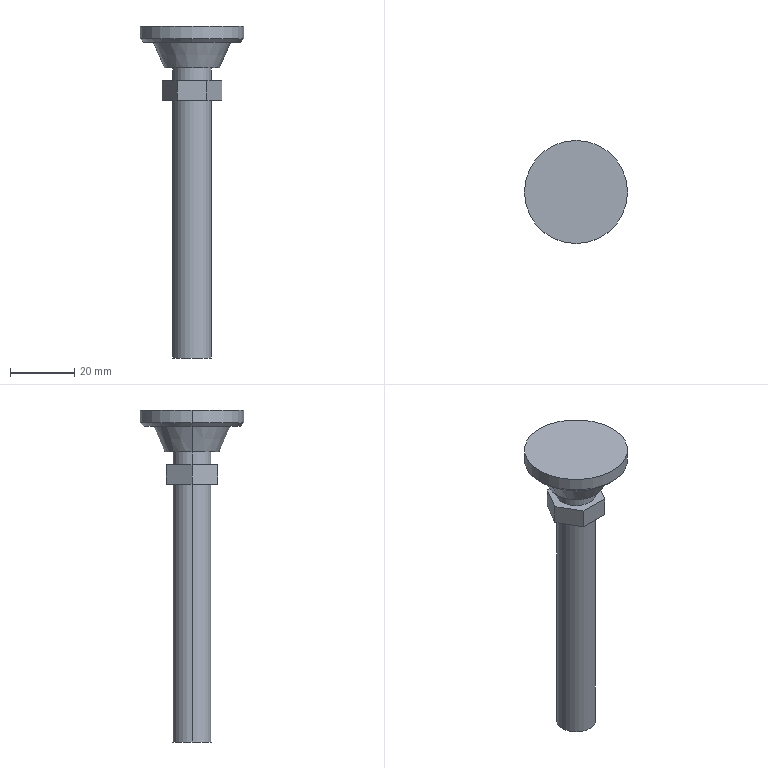Part | STEP file | 274D2D3-1.stp.STEP | 2 solids | 27 faces | box 32 x 32 x 103 mm | volume 17446 mm3 | plane 12 | cylinder 6 | cone 5 | sphere 4 | commonest cylinder face diameters 12 x4 32 x2
STEP:
#1=CARTESIAN_POINT('',(-6.1,0.,-13.));
#2=VERTEX_POINT('',#1);
#3=CARTESIAN_POINT('',(6.1,0.,-13.));
#4=VERTEX_POINT('',#3);
#5=CARTESIAN_POINT('',(0.,0.,-13.));
#6=DIRECTION('',(0.,1.,0.));
#7=DIRECTION('',(-1.,0.,0.));
#8=AXIS2_PLACEMENT_3D('',#5,#6,#7);
#9=CIRCLE('',#8,6.1);
#10=EDGE_CURVE('',#2,#4,#9,.T.);
#11=ORIENTED_EDGE('',*,*,#10,.T.);
#12=CARTESIAN_POINT('',(0.,0.,-13.));
#13=DIRECTION('',(0.,0.,-1.));
#14=DIRECTION('',(1.,0.,0.));
#15=AXIS2_PLACEMENT_3D('',#12,#13,#14);
#16=CIRCLE('',#15,6.1);
#17=EDGE_CURVE('',#4,#2,#16,.T.);
#18=ORIENTED_EDGE('',*,*,#17,.T.);
#19=EDGE_LOOP('',(#11,#18));
#20=FACE_OUTER_BOUND('',#19,.T.);
#21=CARTESIAN_POINT('',(0.,0.,-13.));
#22=DIRECTION('',(0.,0.,1.));
#23=DIRECTION('',(1.,0.,0.));
#24=AXIS2_PLACEMENT_3D('',#21,#22,#23);
#25=SPHERICAL_SURFACE('',#24,6.1);
#26=ADVANCED_FACE('',(#20),#25,.F.);
#27=ORIENTED_EDGE('',*,*,#17,.F.);
#28=CARTESIAN_POINT('',(0.,0.,-13.));
#29=DIRECTION('',(0.,0.,-1.));
#30=DIRECTION('',(-1.,0.,0.));
#31=AXIS2_PLACEMENT_3D('',#28,#29,#30);
#32=CIRCLE('',#31,6.1);
#33=EDGE_CURVE('',#2,#4,#32,.T.);
#34=ORIENTED_EDGE('',*,*,#33,.F.);
#35=EDGE_LOOP('',(#27,#34));
#36=FACE_BOUND('',#35,.T.);
#37=CARTESIAN_POINT('',(8.5,0.,-13.));
#38=VERTEX_POINT('',#37);
#39=CARTESIAN_POINT('',(-8.5,0.,-13.));
#40=VERTEX_POINT('',#39);
#41=CARTESIAN_POINT('',(0.,0.,-13.));
#42=DIRECTION('',(0.,0.,-1.));
#43=DIRECTION('',(1.,0.,0.));
#44=AXIS2_PLACEMENT_3D('',#41,#42,#43);
#45=CIRCLE('',#44,8.5);
#46=EDGE_CURVE('',#38,#40,#45,.T.);
#47=ORIENTED_EDGE('',*,*,#46,.T.);
#48=CARTESIAN_POINT('',(0.,0.,-13.));
#49=DIRECTION('',(0.,0.,1.));
#50=DIRECTION('',(1.,0.,0.));
#51=AXIS2_PLACEMENT_3D('',#48,#49,#50);
#52=CIRCLE('',#51,8.5);
#53=EDGE_CURVE('',#38,#40,#52,.T.);
#54=ORIENTED_EDGE('',*,*,#53,.F.);
#55=EDGE_LOOP('',(#47,#54));
#56=FACE_OUTER_BOUND('',#55,.T.);
#57=CARTESIAN_POINT('',(0.,0.,-13.));
#58=DIRECTION('',(0.,0.,1.));
#59=DIRECTION('',(1.,0.,0.));
#60=AXIS2_PLACEMENT_3D('',#57,#58,#59);
#61=PLANE('',#60);
#62=ADVANCED_FACE('',(#36,#56),#61,.F.);
#63=ORIENTED_EDGE('',*,*,#53,.T.);
#64=CARTESIAN_POINT('',(-12.,0.,-5.));
#65=VERTEX_POINT('',#64);
#66=CARTESIAN_POINT('',(-12.,0.,-5.));
#67=DIRECTION('',(0.4008,0.,-0.9162));
#68=VECTOR('',#67,1000.);
#69=LINE('',#66,#68);
#70=EDGE_CURVE('',#65,#40,#69,.T.);
#71=ORIENTED_EDGE('',*,*,#70,.F.);
#72=CARTESIAN_POINT('',(12.,0.,-5.));
#73=VERTEX_POINT('',#72);
#74=CARTESIAN_POINT('',(0.,0.,-5.));
#75=DIRECTION('',(0.,0.,1.));
#76=DIRECTION('',(1.,0.,0.));
#77=AXIS2_PLACEMENT_3D('',#74,#75,#76);
#78=CIRCLE('',#77,12.);
#79=EDGE_CURVE('',#73,#65,#78,.T.);
#80=ORIENTED_EDGE('',*,*,#79,.F.);
#81=CARTESIAN_POINT('',(12.,0.,-5.));
#82=DIRECTION('',(-0.4008,0.,-0.9162));
#83=VECTOR('',#82,1000.);
#84=LINE('',#81,#83);
#85=EDGE_CURVE('',#73,#38,#84,.T.);
#86=ORIENTED_EDGE('',*,*,#85,.T.);
#87=EDGE_LOOP('',(#63,#71,#80,#86));
#88=FACE_OUTER_BOUND('',#87,.T.);
#89=CARTESIAN_POINT('',(0.,0.,-9.));
#90=DIRECTION('',(0.,0.,1.));
#91=DIRECTION('',(-1.,0.,0.));
#92=AXIS2_PLACEMENT_3D('',#89,#90,#91);
#93=CONICAL_SURFACE('',#92,10.25,0.4124);
#94=ADVANCED_FACE('',(#88),#93,.T.);
#95=CARTESIAN_POINT('',(0.,0.,-5.));
#96=DIRECTION('',(0.,0.,-1.));
#97=DIRECTION('',(1.,0.,0.));
#98=AXIS2_PLACEMENT_3D('',#95,#96,#97);
#99=CIRCLE('',#98,12.);
#100=EDGE_CURVE('',#73,#65,#99,.T.);
#101=ORIENTED_EDGE('',*,*,#100,.T.);
#102=ORIENTED_EDGE('',*,*,#70,.T.);
#103=ORIENTED_EDGE('',*,*,#46,.F.);
#104=ORIENTED_EDGE('',*,*,#85,.F.);
#105=EDGE_LOOP('',(#101,#102,#103,#104));
#106=FACE_OUTER_BOUND('',#105,.T.);
#107=CARTESIAN_POINT('',(0.,0.,-9.));
#108=DIRECTION('',(0.,0.,1.));
#109=DIRECTION('',(-1.,0.,0.));
#110=AXIS2_PLACEMENT_3D('',#107,#108,#109);
#111=CONICAL_SURFACE('',#110,10.25,0.4124);
#112=ADVANCED_FACE('',(#106),#111,.T.);
#113=ORIENTED_EDGE('',*,*,#79,.T.);
#114=ORIENTED_EDGE('',*,*,#100,.F.);
#115=EDGE_LOOP('',(#113,#114));
#116=FACE_BOUND('',#115,.T.);
#117=CARTESIAN_POINT('',(15.,0.,-5.));
#118=VERTEX_POINT('',#117);
#119=CARTESIAN_POINT('',(0.,-15.,-5.));
#120=VERTEX_POINT('',#119);
#121=CARTESIAN_POINT('',(0.,0.,-5.));
#122=DIRECTION('',(0.,0.,-1.));
#123=DIRECTION('',(1.,0.,0.));
#124=AXIS2_PLACEMENT_3D('',#121,#122,#123);
#125=CIRCLE('',#124,15.);
#126=EDGE_CURVE('',#118,#120,#125,.T.);
#127=ORIENTED_EDGE('',*,*,#126,.T.);
#128=CARTESIAN_POINT('',(-15.,0.,-5.));
#129=VERTEX_POINT('',#128);
#130=CARTESIAN_POINT('',(0.,0.,-5.));
#131=DIRECTION('',(0.,0.,-1.));
#132=DIRECTION('',(1.,0.,0.));
#133=AXIS2_PLACEMENT_3D('',#130,#131,#132);
#134=CIRCLE('',#133,15.);
#135=EDGE_CURVE('',#120,#129,#134,.T.);
#136=ORIENTED_EDGE('',*,*,#135,.T.);
#137=CARTESIAN_POINT('',(0.,0.,-5.));
#138=DIRECTION('',(0.,0.,-1.));
#139=DIRECTION('',(-1.,0.,0.));
#140=AXIS2_PLACEMENT_3D('',#137,#138,#139);
#141=CIRCLE('',#140,15.);
#142=EDGE_CURVE('',#129,#118,#141,.T.);
#143=ORIENTED_EDGE('',*,*,#142,.T.);
#144=EDGE_LOOP('',(#127,#136,#143));
#145=FACE_OUTER_BOUND('',#144,.T.);
#146=CARTESIAN_POINT('',(0.,0.,-5.));
#147=DIRECTION('',(0.,0.,1.));
#148=DIRECTION('',(1.,0.,0.));
#149=AXIS2_PLACEMENT_3D('',#146,#147,#148);
#150=PLANE('',#149);
#151=ADVANCED_FACE('',(#116,#145),#150,.F.);
#152=CARTESIAN_POINT('',(-16.,0.,-4.));
#153=VERTEX_POINT('',#152);
#154=CARTESIAN_POINT('',(-15.,-0.000000006,-5.));
#155=DIRECTION('',(-0.7071,0.000000001,0.7071));
#156=VECTOR('',#155,1000.);
#157=LINE('',#154,#156);
#158=EDGE_CURVE('',#129,#153,#157,.T.);
#159=ORIENTED_EDGE('',*,*,#158,.T.);
#160=CARTESIAN_POINT('',(16.,0.,-4.));
#161=VERTEX_POINT('',#160);
#162=CARTESIAN_POINT('',(0.,0.,-4.));
#163=DIRECTION('',(0.,0.,-1.));
#164=DIRECTION('',(-1.,0.,0.));
#165=AXIS2_PLACEMENT_3D('',#162,#163,#164);
#166=CIRCLE('',#165,16.);
#167=EDGE_CURVE('',#153,#161,#166,.T.);
#168=ORIENTED_EDGE('',*,*,#167,.T.);
#169=CARTESIAN_POINT('',(15.,0.000000006,-5.));
#170=DIRECTION('',(0.7071,-0.000000001,0.7071));
#171=VECTOR('',#170,1000.);
#172=LINE('',#169,#171);
#173=EDGE_CURVE('',#118,#161,#172,.T.);
#174=ORIENTED_EDGE('',*,*,#173,.F.);
#175=ORIENTED_EDGE('',*,*,#142,.F.);
#176=EDGE_LOOP('',(#159,#168,#174,#175));
#177=FACE_OUTER_BOUND('',#176,.T.);
#178=CARTESIAN_POINT('',(0.,0.,-4.5));
#179=DIRECTION('',(0.,0.,1.));
#180=DIRECTION('',(0.,-1.,0.));
#181=AXIS2_PLACEMENT_3D('',#178,#179,#180);
#182=CONICAL_SURFACE('',#181,15.5,0.7854);
#183=ADVANCED_FACE('',(#177),#182,.T.);
#184=CARTESIAN_POINT('',(0.,-16.,-4.));
#185=VERTEX_POINT('',#184);
#186=CARTESIAN_POINT('',(0.,-15.5,-4.5));
#187=DIRECTION('',(0.,-0.7071,0.7071));
#188=VECTOR('',#187,1000.);
#189=LINE('',#186,#188);
#190=EDGE_CURVE('',#120,#185,#189,.T.);
#191=ORIENTED_EDGE('',*,*,#190,.F.);
#192=ORIENTED_EDGE('',*,*,#126,.F.);
#193=ORIENTED_EDGE('',*,*,#173,.T.);
#194=CARTESIAN_POINT('',(0.,0.,-4.));
#195=DIRECTION('',(0.,0.,-1.));
#196=DIRECTION('',(1.,0.,0.));
#197=AXIS2_PLACEMENT_3D('',#194,#195,#196);
#198=CIRCLE('',#197,16.);
#199=EDGE_CURVE('',#161,#185,#198,.T.);
#200=ORIENTED_EDGE('',*,*,#199,.T.);
#201=EDGE_LOOP('',(#191,#192,#193,#200));
#202=FACE_OUTER_BOUND('',#201,.T.);
#203=CARTESIAN_POINT('',(0.,0.,-4.5));
#204=DIRECTION('',(0.,0.,1.));
#205=DIRECTION('',(0.,-1.,0.));
#206=AXIS2_PLACEMENT_3D('',#203,#204,#205);
#207=CONICAL_SURFACE('',#206,15.5,0.7854);
#208=ADVANCED_FACE('',(#202),#207,.T.);
#209=CARTESIAN_POINT('',(16.,0.,0.));
#210=VERTEX_POINT('',#209);
#211=CARTESIAN_POINT('',(16.,0.,0.));
#212=DIRECTION('',(0.,0.000000001,-1.));
#213=VECTOR('',#212,1000.);
#214=LINE('',#211,#213);
#215=EDGE_CURVE('',#210,#161,#214,.T.);
#216=ORIENTED_EDGE('',*,*,#215,.F.);
#217=CARTESIAN_POINT('',(-16.,0.,0.));
#218=VERTEX_POINT('',#217);
#219=CARTESIAN_POINT('',(0.,0.,0.));
#220=DIRECTION('',(0.,0.,-1.));
#221=DIRECTION('',(1.,0.,0.));
#222=AXIS2_PLACEMENT_3D('',#219,#220,#221);
#223=CIRCLE('',#222,16.);
#224=EDGE_CURVE('',#210,#218,#223,.T.);
#225=ORIENTED_EDGE('',*,*,#224,.T.);
#226=CARTESIAN_POINT('',(-16.,0.,0.));
#227=DIRECTION('',(0.,-0.000000001,-1.));
#228=VECTOR('',#227,1000.);
#229=LINE('',#226,#228);
#230=EDGE_CURVE('',#218,#153,#229,.T.);
#231=ORIENTED_EDGE('',*,*,#230,.T.);
#232=CARTESIAN_POINT('',(0.,0.,-4.));
#233=DIRECTION('',(0.,0.,-1.));
#234=DIRECTION('',(1.,0.,0.));
#235=AXIS2_PLACEMENT_3D('',#232,#233,#234);
#236=CIRCLE('',#235,16.);
#237=EDGE_CURVE('',#185,#153,#236,.T.);
#238=ORIENTED_EDGE('',*,*,#237,.F.);
#239=ORIENTED_EDGE('',*,*,#199,.F.);
#240=EDGE_LOOP('',(#216,#225,#231,#238,#239));
#241=FACE_OUTER_BOUND('',#240,.T.);
#242=CARTESIAN_POINT('',(0.,0.,-108.15));
#243=DIRECTION('',(0.,0.,1.));
#244=DIRECTION('',(-1.,0.,0.));
#245=AXIS2_PLACEMENT_3D('',#242,#243,#244);
#246=CYLINDRICAL_SURFACE('',#245,16.);
#247=ADVANCED_FACE('',(#241),#246,.T.);
#248=ORIENTED_EDGE('',*,*,#230,.F.);
#249=CARTESIAN_POINT('',(0.,0.,0.));
#250=DIRECTION('',(0.,0.,1.));
#251=DIRECTION('',(1.,0.,0.));
#252=AXIS2_PLACEMENT_3D('',#249,#250,#251);
#253=CIRCLE('',#252,16.);
#254=EDGE_CURVE('',#210,#218,#253,.T.);
#255=ORIENTED_EDGE('',*,*,#254,.F.);
#256=ORIENTED_EDGE('',*,*,#215,.T.);
#257=ORIENTED_EDGE('',*,*,#167,.F.);
#258=EDGE_LOOP('',(#248,#255,#256,#257));
#259=FACE_OUTER_BOUND('',#258,.T.);
#260=CARTESIAN_POINT('',(0.,0.,-108.15));
#261=DIRECTION('',(0.,0.,1.));
#262=DIRECTION('',(-1.,0.,0.));
#263=AXIS2_PLACEMENT_3D('',#260,#261,#262);
#264=CYLINDRICAL_SURFACE('',#263,16.);
#265=ADVANCED_FACE('',(#259),#264,.T.);
#266=ORIENTED_EDGE('',*,*,#254,.T.);
#267=ORIENTED_EDGE('',*,*,#224,.F.);
#268=EDGE_LOOP('',(#266,#267));
#269=FACE_OUTER_BOUND('',#268,.T.);
#270=CARTESIAN_POINT('',(0.,0.,0.));
#271=DIRECTION('',(0.,0.,1.));
#272=DIRECTION('',(1.,0.,0.));
#273=AXIS2_PLACEMENT_3D('',#270,#271,#272);
#274=PLANE('',#273);
#275=ADVANCED_FACE('',(#269),#274,.T.);
#276=ORIENTED_EDGE('',*,*,#33,.T.);
#277=ORIENTED_EDGE('',*,*,#10,.F.);
#278=EDGE_LOOP('',(#276,#277));
#279=FACE_OUTER_BOUND('',#278,.T.);
#280=CARTESIAN_POINT('',(0.,0.,-13.));
#281=DIRECTION('',(0.,0.,1.));
#282=DIRECTION('',(1.,0.,0.));
#283=AXIS2_PLACEMENT_3D('',#280,#281,#282);
#284=SPHERICAL_SURFACE('',#283,6.1);
#285=ADVANCED_FACE('',(#279),#284,.F.);
#286=ORIENTED_EDGE('',*,*,#135,.F.);
#287=ORIENTED_EDGE('',*,*,#190,.T.);
#288=ORIENTED_EDGE('',*,*,#237,.T.);
#289=ORIENTED_EDGE('',*,*,#158,.F.);
#290=EDGE_LOOP('',(#286,#287,#288,#289));
#291=FACE_OUTER_BOUND('',#290,.T.);
#292=CARTESIAN_POINT('',(0.,0.,-4.5));
#293=DIRECTION('',(0.,0.,1.));
#294=DIRECTION('',(0.,-1.,0.));
#295=AXIS2_PLACEMENT_3D('',#292,#293,#294);
#296=CONICAL_SURFACE('',#295,15.5,0.7854);
#297=ADVANCED_FACE('',(#291),#296,.T.);
#298=CLOSED_SHELL('',(#26,#62,#94,#112,#151,#183,#208,#247,#265,#275,#285,#297));
#299=MANIFOLD_SOLID_BREP('',#298);
#300=CARTESIAN_POINT('',(-6.,0.,-13.));
#301=VERTEX_POINT('',#300);
#302=CARTESIAN_POINT('',(6.,0.,-13.));
#303=VERTEX_POINT('',#302);
#304=CARTESIAN_POINT('',(0.,0.,-13.));
#305=DIRECTION('',(0.,1.,0.));
#306=DIRECTION('',(0.,0.,1.));
#307=AXIS2_PLACEMENT_3D('',#304,#305,#306);
#308=CIRCLE('',#307,6.);
#309=EDGE_CURVE('',#301,#303,#308,.T.);
#310=ORIENTED_EDGE('',*,*,#309,.F.);
#311=CARTESIAN_POINT('',(0.,0.,-13.));
#312=DIRECTION('',(0.,0.,-1.));
#313=DIRECTION('',(1.,0.,0.));
#314=AXIS2_PLACEMENT_3D('',#311,#312,#313);
#315=CIRCLE('',#314,6.);
#316=EDGE_CURVE('',#303,#301,#315,.T.);
#317=ORIENTED_EDGE('',*,*,#316,.F.);
#318=EDGE_LOOP('',(#310,#317));
#319=FACE_OUTER_BOUND('',#318,.T.);
#320=CARTESIAN_POINT('',(0.,0.,-13.));
#321=DIRECTION('',(0.,0.,1.));
#322=DIRECTION('',(1.,0.,0.));
#323=AXIS2_PLACEMENT_3D('',#320,#321,#322);
#324=SPHERICAL_SURFACE('',#323,6.);
#325=ADVANCED_FACE('',(#319),#324,.T.);
#326=CARTESIAN_POINT('',(-6.,0.,-23.));
#327=VERTEX_POINT('',#326);
#328=CARTESIAN_POINT('',(-6.,0.,-103.));
#329=VERTEX_POINT('',#328);
#330=CARTESIAN_POINT('',(-6.,0.,-23.));
#331=DIRECTION('',(0.,0.,-1.));
#332=VECTOR('',#331,1000.);
#333=LINE('',#330,#332);
#334=EDGE_CURVE('',#327,#329,#333,.T.);
#335=ORIENTED_EDGE('',*,*,#334,.T.);
#336=CARTESIAN_POINT('',(6.,0.,-103.));
#337=VERTEX_POINT('',#336);
#338=CARTESIAN_POINT('',(0.,0.,-103.));
#339=DIRECTION('',(0.,0.,-1.));
#340=DIRECTION('',(1.,0.,0.));
#341=AXIS2_PLACEMENT_3D('',#338,#339,#340);
#342=CIRCLE('',#341,6.);
#343=EDGE_CURVE('',#337,#329,#342,.T.);
#344=ORIENTED_EDGE('',*,*,#343,.F.);
#345=CARTESIAN_POINT('',(6.,0.,-23.));
#346=VERTEX_POINT('',#345);
#347=CARTESIAN_POINT('',(6.,0.,-23.));
#348=DIRECTION('',(0.,0.,-1.));
#349=VECTOR('',#348,1000.);
#350=LINE('',#347,#349);
#351=EDGE_CURVE('',#346,#337,#350,.T.);
#352=ORIENTED_EDGE('',*,*,#351,.F.);
#353=CARTESIAN_POINT('',(0.,0.,-23.));
#354=DIRECTION('',(0.,0.,1.));
#355=DIRECTION('',(-1.,0.,0.));
#356=AXIS2_PLACEMENT_3D('',#353,#354,#355);
#357=CIRCLE('',#356,6.);
#358=EDGE_CURVE('',#327,#346,#357,.T.);
#359=ORIENTED_EDGE('',*,*,#358,.F.);
#360=EDGE_LOOP('',(#335,#344,#352,#359));
#361=FACE_OUTER_BOUND('',#360,.T.);
#362=CARTESIAN_POINT('',(0.,0.,-108.15));
#363=DIRECTION('',(0.,0.,1.));
#364=DIRECTION('',(-1.,0.,0.));
#365=AXIS2_PLACEMENT_3D('',#362,#363,#364);
#366=CYLINDRICAL_SURFACE('',#365,6.);
#367=ADVANCED_FACE('',(#361),#366,.T.);
#368=ORIENTED_EDGE('',*,*,#316,.T.);
#369=CARTESIAN_POINT('',(-6.,0.,-17.));
#370=VERTEX_POINT('',#369);
#371=CARTESIAN_POINT('',(-6.,0.,-13.));
#372=DIRECTION('',(0.,0.,-1.));
#373=VECTOR('',#372,1000.);
#374=LINE('',#371,#373);
#375=EDGE_CURVE('',#301,#370,#374,.T.);
#376=ORIENTED_EDGE('',*,*,#375,.T.);
#377=CARTESIAN_POINT('',(6.,0.,-17.));
#378=VERTEX_POINT('',#377);
#379=CARTESIAN_POINT('',(0.,0.,-17.));
#380=DIRECTION('',(0.,0.,-1.));
#381=DIRECTION('',(1.,0.,0.));
#382=AXIS2_PLACEMENT_3D('',#379,#380,#381);
#383=CIRCLE('',#382,6.);
#384=EDGE_CURVE('',#378,#370,#383,.T.);
#385=ORIENTED_EDGE('',*,*,#384,.F.);
#386=CARTESIAN_POINT('',(6.,0.,-13.));
#387=DIRECTION('',(0.,0.,-1.));
#388=VECTOR('',#387,1000.);
#389=LINE('',#386,#388);
#390=EDGE_CURVE('',#303,#378,#389,.T.);
#391=ORIENTED_EDGE('',*,*,#390,.F.);
#392=EDGE_LOOP('',(#368,#376,#385,#391));
#393=FACE_OUTER_BOUND('',#392,.T.);
#394=CARTESIAN_POINT('',(0.,0.,-108.15));
#395=DIRECTION('',(0.,0.,1.));
#396=DIRECTION('',(-1.,0.,0.));
#397=AXIS2_PLACEMENT_3D('',#394,#395,#396);
#398=CYLINDRICAL_SURFACE('',#397,6.);
#399=ADVANCED_FACE('',(#393),#398,.T.);
#400=ORIENTED_EDGE('',*,*,#358,.T.);
#401=CARTESIAN_POINT('',(0.,0.,-23.));
#402=DIRECTION('',(0.,0.,1.));
#403=DIRECTION('',(1.,0.,0.));
#404=AXIS2_PLACEMENT_3D('',#401,#402,#403);
#405=CIRCLE('',#404,6.);
#406=EDGE_CURVE('',#346,#327,#405,.T.);
#407=ORIENTED_EDGE('',*,*,#406,.T.);
#408=EDGE_LOOP('',(#400,#407));
#409=FACE_BOUND('',#408,.T.);
#410=CARTESIAN_POINT('',(-9.238,0.,-23.));
#411=VERTEX_POINT('',#410);
#412=CARTESIAN_POINT('',(-4.619,8.,-23.));
#413=VERTEX_POINT('',#412);
#414=CARTESIAN_POINT('',(-9.238,0.,-23.));
#415=DIRECTION('',(0.5,0.866,0.));
#416=VECTOR('',#415,1000.);
#417=LINE('',#414,#416);
#418=EDGE_CURVE('',#411,#413,#417,.T.);
#419=ORIENTED_EDGE('',*,*,#418,.T.);
#420=CARTESIAN_POINT('',(4.619,8.,-23.));
#421=VERTEX_POINT('',#420);
#422=CARTESIAN_POINT('',(-4.619,8.,-23.));
#423=DIRECTION('',(1.,0.,0.));
#424=VECTOR('',#423,1000.);
#425=LINE('',#422,#424);
#426=EDGE_CURVE('',#413,#421,#425,.T.);
#427=ORIENTED_EDGE('',*,*,#426,.T.);
#428=CARTESIAN_POINT('',(9.238,0.,-23.));
#429=VERTEX_POINT('',#428);
#430=CARTESIAN_POINT('',(4.619,8.,-23.));
#431=DIRECTION('',(0.5,-0.866,0.));
#432=VECTOR('',#431,1000.);
#433=LINE('',#430,#432);
#434=EDGE_CURVE('',#421,#429,#433,.T.);
#435=ORIENTED_EDGE('',*,*,#434,.T.);
#436=CARTESIAN_POINT('',(4.619,-8.,-23.));
#437=VERTEX_POINT('',#436);
#438=CARTESIAN_POINT('',(9.238,0.,-23.));
#439=DIRECTION('',(-0.5,-0.866,0.));
#440=VECTOR('',#439,1000.);
#441=LINE('',#438,#440);
#442=EDGE_CURVE('',#429,#437,#441,.T.);
#443=ORIENTED_EDGE('',*,*,#442,.T.);
#444=CARTESIAN_POINT('',(-4.619,-8.,-23.));
#445=VERTEX_POINT('',#444);
#446=CARTESIAN_POINT('',(4.619,-8.,-23.));
#447=DIRECTION('',(-1.,0.,0.));
#448=VECTOR('',#447,1000.);
#449=LINE('',#446,#448);
#450=EDGE_CURVE('',#437,#445,#449,.T.);
#451=ORIENTED_EDGE('',*,*,#450,.T.);
#452=CARTESIAN_POINT('',(-4.619,-8.,-23.));
#453=DIRECTION('',(-0.5,0.866,0.));
#454=VECTOR('',#453,1000.);
#455=LINE('',#452,#454);
#456=EDGE_CURVE('',#445,#411,#455,.T.);
#457=ORIENTED_EDGE('',*,*,#456,.T.);
#458=EDGE_LOOP('',(#419,#427,#435,#443,#451,#457));
#459=FACE_OUTER_BOUND('',#458,.T.);
#460=CARTESIAN_POINT('',(0.,0.,-23.));
#461=DIRECTION('',(0.,0.,1.));
#462=DIRECTION('',(1.,0.,0.));
#463=AXIS2_PLACEMENT_3D('',#460,#461,#462);
#464=PLANE('',#463);
#465=ADVANCED_FACE('',(#409,#459),#464,.F.);
#466=CARTESIAN_POINT('',(-4.619,-8.,-17.));
#467=VERTEX_POINT('',#466);
#468=CARTESIAN_POINT('',(-4.619,-8.,-17.));
#469=DIRECTION('',(0.,0.,-1.));
#470=VECTOR('',#469,1000.);
#471=LINE('',#468,#470);
#472=EDGE_CURVE('',#467,#445,#471,.T.);
#473=ORIENTED_EDGE('',*,*,#472,.F.);
#474=CARTESIAN_POINT('',(-9.238,0.,-17.));
#475=VERTEX_POINT('',#474);
#476=CARTESIAN_POINT('',(-4.619,-8.,-17.));
#477=DIRECTION('',(-0.5,0.866,0.));
#478=VECTOR('',#477,1000.);
#479=LINE('',#476,#478);
#480=EDGE_CURVE('',#467,#475,#479,.T.);
#481=ORIENTED_EDGE('',*,*,#480,.T.);
#482=CARTESIAN_POINT('',(-9.238,0.,-17.));
#483=DIRECTION('',(0.,0.,-1.));
#484=VECTOR('',#483,1000.);
#485=LINE('',#482,#484);
#486=EDGE_CURVE('',#475,#411,#485,.T.);
#487=ORIENTED_EDGE('',*,*,#486,.T.);
#488=ORIENTED_EDGE('',*,*,#456,.F.);
#489=EDGE_LOOP('',(#473,#481,#487,#488));
#490=FACE_OUTER_BOUND('',#489,.T.);
#491=CARTESIAN_POINT('',(-9.238,0.,-23.));
#492=DIRECTION('',(-0.866,-0.5,0.));
#493=DIRECTION('',(-0.5,0.866,0.));
#494=AXIS2_PLACEMENT_3D('',#491,#492,#493);
#495=PLANE('',#494);
#496=ADVANCED_FACE('',(#490),#495,.T.);
#497=ORIENTED_EDGE('',*,*,#486,.F.);
#498=CARTESIAN_POINT('',(-4.619,8.,-17.));
#499=VERTEX_POINT('',#498);
#500=CARTESIAN_POINT('',(-9.238,0.,-17.));
#501=DIRECTION('',(0.5,0.866,0.));
#502=VECTOR('',#501,1000.);
#503=LINE('',#500,#502);
#504=EDGE_CURVE('',#475,#499,#503,.T.);
#505=ORIENTED_EDGE('',*,*,#504,.T.);
#506=CARTESIAN_POINT('',(-4.619,8.,-17.));
#507=DIRECTION('',(0.,0.,-1.));
#508=VECTOR('',#507,1000.);
#509=LINE('',#506,#508);
#510=EDGE_CURVE('',#499,#413,#509,.T.);
#511=ORIENTED_EDGE('',*,*,#510,.T.);
#512=ORIENTED_EDGE('',*,*,#418,.F.);
#513=EDGE_LOOP('',(#497,#505,#511,#512));
#514=FACE_OUTER_BOUND('',#513,.T.);
#515=CARTESIAN_POINT('',(-4.619,8.,-23.));
#516=DIRECTION('',(-0.866,0.5,0.));
#517=DIRECTION('',(0.,0.,1.));
#518=AXIS2_PLACEMENT_3D('',#515,#516,#517);
#519=PLANE('',#518);
#520=ADVANCED_FACE('',(#514),#519,.T.);
#521=ORIENTED_EDGE('',*,*,#510,.F.);
#522=CARTESIAN_POINT('',(4.619,8.,-17.));
#523=VERTEX_POINT('',#522);
#524=CARTESIAN_POINT('',(-4.619,8.,-17.));
#525=DIRECTION('',(1.,0.,0.));
#526=VECTOR('',#525,1000.);
#527=LINE('',#524,#526);
#528=EDGE_CURVE('',#499,#523,#527,.T.);
#529=ORIENTED_EDGE('',*,*,#528,.T.);
#530=CARTESIAN_POINT('',(4.619,8.,-17.));
#531=DIRECTION('',(0.,0.,-1.));
#532=VECTOR('',#531,1000.);
#533=LINE('',#530,#532);
#534=EDGE_CURVE('',#523,#421,#533,.T.);
#535=ORIENTED_EDGE('',*,*,#534,.T.);
#536=ORIENTED_EDGE('',*,*,#426,.F.);
#537=EDGE_LOOP('',(#521,#529,#535,#536));
#538=FACE_OUTER_BOUND('',#537,.T.);
#539=CARTESIAN_POINT('',(4.619,8.,-23.));
#540=DIRECTION('',(0.,1.,0.));
#541=DIRECTION('',(1.,0.,0.));
#542=AXIS2_PLACEMENT_3D('',#539,#540,#541);
#543=PLANE('',#542);
#544=ADVANCED_FACE('',(#538),#543,.T.);
#545=ORIENTED_EDGE('',*,*,#534,.F.);
#546=CARTESIAN_POINT('',(9.238,0.,-17.));
#547=VERTEX_POINT('',#546);
#548=CARTESIAN_POINT('',(4.619,8.,-17.));
#549=DIRECTION('',(0.5,-0.866,0.));
#550=VECTOR('',#549,1000.);
#551=LINE('',#548,#550);
#552=EDGE_CURVE('',#523,#547,#551,.T.);
#553=ORIENTED_EDGE('',*,*,#552,.T.);
#554=CARTESIAN_POINT('',(9.238,0.,-17.));
#555=DIRECTION('',(0.,0.,-1.));
#556=VECTOR('',#555,1000.);
#557=LINE('',#554,#556);
#558=EDGE_CURVE('',#547,#429,#557,.T.);
#559=ORIENTED_EDGE('',*,*,#558,.T.);
#560=ORIENTED_EDGE('',*,*,#434,.F.);
#561=EDGE_LOOP('',(#545,#553,#559,#560));
#562=FACE_OUTER_BOUND('',#561,.T.);
#563=CARTESIAN_POINT('',(9.238,0.,-23.));
#564=DIRECTION('',(0.866,0.5,0.));
#565=DIRECTION('',(0.,0.,-1.));
#566=AXIS2_PLACEMENT_3D('',#563,#564,#565);
#567=PLANE('',#566);
#568=ADVANCED_FACE('',(#562),#567,.T.);
#569=ORIENTED_EDGE('',*,*,#558,.F.);
#570=CARTESIAN_POINT('',(4.619,-8.,-17.));
#571=VERTEX_POINT('',#570);
#572=CARTESIAN_POINT('',(9.238,0.,-17.));
#573=DIRECTION('',(-0.5,-0.866,0.));
#574=VECTOR('',#573,1000.);
#575=LINE('',#572,#574);
#576=EDGE_CURVE('',#547,#571,#575,.T.);
#577=ORIENTED_EDGE('',*,*,#576,.T.);
#578=CARTESIAN_POINT('',(4.619,-8.,-17.));
#579=DIRECTION('',(0.,0.,-1.));
#580=VECTOR('',#579,1000.);
#581=LINE('',#578,#580);
#582=EDGE_CURVE('',#571,#437,#581,.T.);
#583=ORIENTED_EDGE('',*,*,#582,.T.);
#584=ORIENTED_EDGE('',*,*,#442,.F.);
#585=EDGE_LOOP('',(#569,#577,#583,#584));
#586=FACE_OUTER_BOUND('',#585,.T.);
#587=CARTESIAN_POINT('',(4.619,-8.,-23.));
#588=DIRECTION('',(0.866,-0.5,0.));
#589=DIRECTION('',(0.,0.,-1.));
#590=AXIS2_PLACEMENT_3D('',#587,#588,#589);
#591=PLANE('',#590);
#592=ADVANCED_FACE('',(#586),#591,.T.);
#593=ORIENTED_EDGE('',*,*,#582,.F.);
#594=CARTESIAN_POINT('',(4.619,-8.,-17.));
#595=DIRECTION('',(-1.,0.,0.));
#596=VECTOR('',#595,1000.);
#597=LINE('',#594,#596);
#598=EDGE_CURVE('',#571,#467,#597,.T.);
#599=ORIENTED_EDGE('',*,*,#598,.T.);
#600=ORIENTED_EDGE('',*,*,#472,.T.);
#601=ORIENTED_EDGE('',*,*,#450,.F.);
#602=EDGE_LOOP('',(#593,#599,#600,#601));
#603=FACE_OUTER_BOUND('',#602,.T.);
#604=CARTESIAN_POINT('',(-4.619,-8.,-23.));
#605=DIRECTION('',(0.,-1.,0.));
#606=DIRECTION('',(0.,0.,-1.));
#607=AXIS2_PLACEMENT_3D('',#604,#605,#606);
#608=PLANE('',#607);
#609=ADVANCED_FACE('',(#603),#608,.T.);
#610=ORIENTED_EDGE('',*,*,#384,.T.);
#611=CARTESIAN_POINT('',(0.,0.,-17.));
#612=DIRECTION('',(0.,0.,-1.));
#613=DIRECTION('',(-1.,0.,0.));
#614=AXIS2_PLACEMENT_3D('',#611,#612,#613);
#615=CIRCLE('',#614,6.);
#616=EDGE_CURVE('',#370,#378,#615,.T.);
#617=ORIENTED_EDGE('',*,*,#616,.T.);
#618=EDGE_LOOP('',(#610,#617));
#619=FACE_BOUND('',#618,.T.);
#620=ORIENTED_EDGE('',*,*,#598,.F.);
#621=ORIENTED_EDGE('',*,*,#576,.F.);
#622=ORIENTED_EDGE('',*,*,#552,.F.);
#623=ORIENTED_EDGE('',*,*,#528,.F.);
#624=ORIENTED_EDGE('',*,*,#504,.F.);
#625=ORIENTED_EDGE('',*,*,#480,.F.);
#626=EDGE_LOOP('',(#620,#621,#622,#623,#624,#625));
#627=FACE_OUTER_BOUND('',#626,.T.);
#628=CARTESIAN_POINT('',(0.,0.,-17.));
#629=DIRECTION('',(0.,0.,1.));
#630=DIRECTION('',(1.,0.,0.));
#631=AXIS2_PLACEMENT_3D('',#628,#629,#630);
#632=PLANE('',#631);
#633=ADVANCED_FACE('',(#619,#627),#632,.T.);
#634=ORIENTED_EDGE('',*,*,#351,.T.);
#635=CARTESIAN_POINT('',(0.,0.,-103.));
#636=DIRECTION('',(0.,0.,1.));
#637=DIRECTION('',(1.,0.,0.));
#638=AXIS2_PLACEMENT_3D('',#635,#636,#637);
#639=CIRCLE('',#638,6.);
#640=EDGE_CURVE('',#337,#329,#639,.T.);
#641=ORIENTED_EDGE('',*,*,#640,.T.);
#642=ORIENTED_EDGE('',*,*,#334,.F.);
#643=ORIENTED_EDGE('',*,*,#406,.F.);
#644=EDGE_LOOP('',(#634,#641,#642,#643));
#645=FACE_OUTER_BOUND('',#644,.T.);
#646=CARTESIAN_POINT('',(0.,0.,-108.15));
#647=DIRECTION('',(0.,0.,1.));
#648=DIRECTION('',(-1.,0.,0.));
#649=AXIS2_PLACEMENT_3D('',#646,#647,#648);
#650=CYLINDRICAL_SURFACE('',#649,6.);
#651=ADVANCED_FACE('',(#645),#650,.T.);
#652=CARTESIAN_POINT('',(0.,0.,-13.));
#653=DIRECTION('',(0.,0.,-1.));
#654=DIRECTION('',(-1.,0.,0.));
#655=AXIS2_PLACEMENT_3D('',#652,#653,#654);
#656=CIRCLE('',#655,6.);
#657=EDGE_CURVE('',#301,#303,#656,.T.);
#658=ORIENTED_EDGE('',*,*,#657,.T.);
#659=ORIENTED_EDGE('',*,*,#390,.T.);
#660=ORIENTED_EDGE('',*,*,#616,.F.);
#661=ORIENTED_EDGE('',*,*,#375,.F.);
#662=EDGE_LOOP('',(#658,#659,#660,#661));
#663=FACE_OUTER_BOUND('',#662,.T.);
#664=CARTESIAN_POINT('',(0.,0.,-108.15));
#665=DIRECTION('',(0.,0.,1.));
#666=DIRECTION('',(-1.,0.,0.));
#667=AXIS2_PLACEMENT_3D('',#664,#665,#666);
#668=CYLINDRICAL_SURFACE('',#667,6.);
#669=ADVANCED_FACE('',(#663),#668,.T.);
#670=ORIENTED_EDGE('',*,*,#640,.F.);
#671=ORIENTED_EDGE('',*,*,#343,.T.);
#672=EDGE_LOOP('',(#670,#671));
#673=FACE_OUTER_BOUND('',#672,.T.);
#674=CARTESIAN_POINT('',(0.,0.,-103.));
#675=DIRECTION('',(0.,0.,1.));
#676=DIRECTION('',(1.,0.,0.));
#677=AXIS2_PLACEMENT_3D('',#674,#675,#676);
#678=PLANE('',#677);
#679=ADVANCED_FACE('',(#673),#678,.F.);
#680=ORIENTED_EDGE('',*,*,#657,.F.);
#681=ORIENTED_EDGE('',*,*,#309,.T.);
#682=EDGE_LOOP('',(#680,#681));
#683=FACE_OUTER_BOUND('',#682,.T.);
#684=CARTESIAN_POINT('',(0.,0.,-13.));
#685=DIRECTION('',(0.,0.,1.));
#686=DIRECTION('',(1.,0.,0.));
#687=AXIS2_PLACEMENT_3D('',#684,#685,#686);
#688=SPHERICAL_SURFACE('',#687,6.);
#689=ADVANCED_FACE('',(#683),#688,.T.);
#690=CLOSED_SHELL('',(#325,#367,#399,#465,#496,#520,#544,#568,#592,#609,#633,#651,#669,#679,#689));
#691=MANIFOLD_SOLID_BREP('',#690);
#692=CARTESIAN_POINT('',(0.,0.,0.));
#693=DIRECTION('',(0.,0.,1.));
#694=DIRECTION('',(1.,0.,0.));
#695=AXIS2_PLACEMENT_3D('',#692,#693,#694);
#696=(LENGTH_UNIT()NAMED_UNIT(*)SI_UNIT(.MILLI.,.METRE.));
#697=UNCERTAINTY_MEASURE_WITH_UNIT(LENGTH_MEASURE(0.00001),#696,'','');
#698=(NAMED_UNIT(*)PLANE_ANGLE_UNIT()SI_UNIT($,.RADIAN.));
#699=(NAMED_UNIT(*)SI_UNIT($,.STERADIAN.)SOLID_ANGLE_UNIT());
#700=(GEOMETRIC_REPRESENTATION_CONTEXT(3)GLOBAL_UNCERTAINTY_ASSIGNED_CONTEXT((#697))GLOBAL_UNIT_ASSIGNED_CONTEXT((#696,#698,#699))REPRESENTATION_CONTEXT('',''));
#701=ADVANCED_BREP_SHAPE_REPRESENTATION('',(#299,#691,#695),#700);